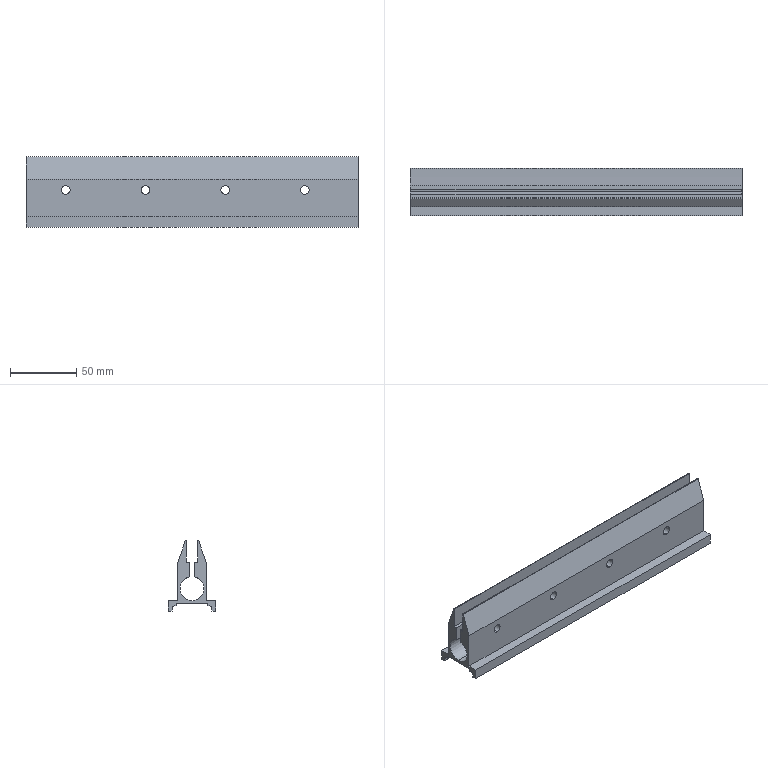Part | STEP file | Blade clamp | 1 solid | 61 faces | box 250 x 36 x 53 mm | volume 139062 mm3 | plane 31 | cylinder 30 | commonest cylinder face diameters 6.5 x16 10.5 x8 2 x2 4 x2 18 x2